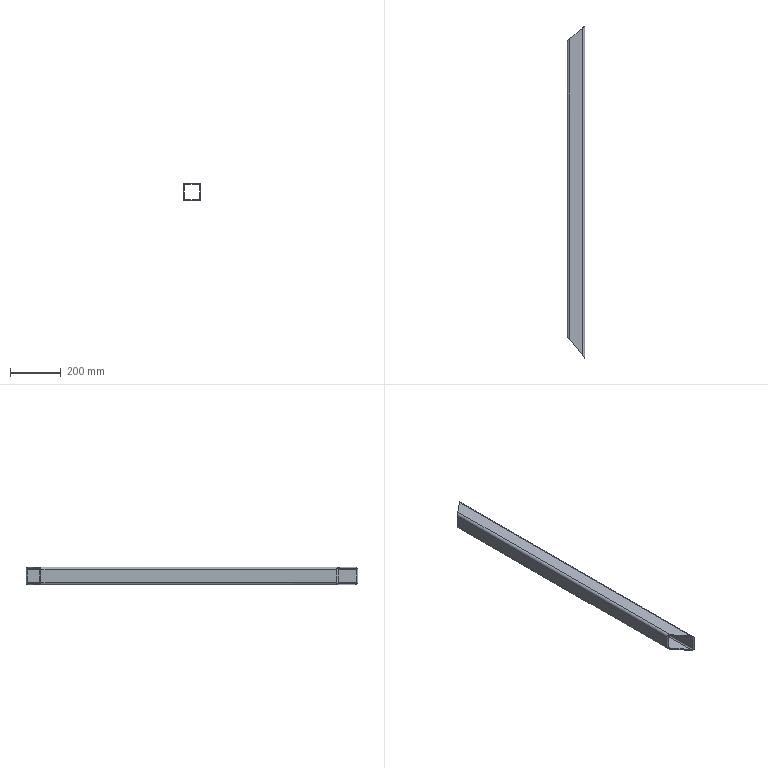Part | SolidWorks | features ICE 1, WeldMemberFeat 1, WeldmentFeature 1 | 1 solid | 18 faces | box 70 x 1302 x 70 mm | volume 1520953 mm3 | plane 10 | cylinder 8 | commonest cylinder face diameters 10 x4 20 x4
STEP:
#1=CARTESIAN_POINT('',(35.,0.,25.));
#2=VERTEX_POINT('',#1);
#3=CARTESIAN_POINT('',(35.,0.,-25.));
#4=VERTEX_POINT('',#3);
#5=CARTESIAN_POINT('',(35.,0.,-25.));
#6=DIRECTION('',(0.,0.,-1.));
#7=VECTOR('',#6,1000.);
#8=LINE('',#5,#7);
#9=EDGE_CURVE('',#2,#4,#8,.T.);
#10=ORIENTED_EDGE('',*,*,#9,.T.);
#11=CARTESIAN_POINT('',(35.,1302.,-25.));
#12=VERTEX_POINT('',#11);
#13=CARTESIAN_POINT('',(35.,1302.,-25.));
#14=DIRECTION('',(0.,-1.,0.));
#15=VECTOR('',#14,1000.);
#16=LINE('',#13,#15);
#17=EDGE_CURVE('',#12,#4,#16,.T.);
#18=ORIENTED_EDGE('',*,*,#17,.F.);
#19=CARTESIAN_POINT('',(35.,1302.,25.));
#20=VERTEX_POINT('',#19);
#21=CARTESIAN_POINT('',(35.,1302.,-25.));
#22=DIRECTION('',(0.,0.,-1.));
#23=VECTOR('',#22,1000.);
#24=LINE('',#21,#23);
#25=EDGE_CURVE('',#20,#12,#24,.T.);
#26=ORIENTED_EDGE('',*,*,#25,.F.);
#27=CARTESIAN_POINT('',(35.,1302.,25.));
#28=DIRECTION('',(0.,-1.,0.));
#29=VECTOR('',#28,1000.);
#30=LINE('',#27,#29);
#31=EDGE_CURVE('',#20,#2,#30,.T.);
#32=ORIENTED_EDGE('',*,*,#31,.T.);
#33=EDGE_LOOP('',(#10,#18,#26,#32));
#34=FACE_OUTER_BOUND('',#33,.T.);
#35=CARTESIAN_POINT('',(35.,1302.,-25.));
#36=DIRECTION('',(-1.,0.,0.));
#37=DIRECTION('',(0.,0.,1.));
#38=AXIS2_PLACEMENT_3D('',#35,#36,#37);
#39=PLANE('',#38);
#40=ADVANCED_FACE('',(#34),#39,.F.);
#41=CARTESIAN_POINT('',(-35.,1243.247,25.));
#42=VERTEX_POINT('',#41);
#43=CARTESIAN_POINT('',(-35.,83.4,25.));
#44=VERTEX_POINT('',#43);
#45=CARTESIAN_POINT('',(-35.,1302.,25.));
#46=DIRECTION('',(0.,-1.,0.));
#47=VECTOR('',#46,1000.);
#48=LINE('',#45,#47);
#49=EDGE_CURVE('',#42,#44,#48,.T.);
#50=ORIENTED_EDGE('',*,*,#49,.F.);
#51=CARTESIAN_POINT('',(-35.,1243.247,-25.));
#52=VERTEX_POINT('',#51);
#53=CARTESIAN_POINT('',(-35.,1243.247,-35.));
#54=DIRECTION('',(0.,0.,1.));
#55=VECTOR('',#54,1000.);
#56=LINE('',#53,#55);
#57=EDGE_CURVE('',#52,#42,#56,.T.);
#58=ORIENTED_EDGE('',*,*,#57,.F.);
#59=CARTESIAN_POINT('',(-35.,83.4,-25.));
#60=VERTEX_POINT('',#59);
#61=CARTESIAN_POINT('',(-35.,1302.,-25.));
#62=DIRECTION('',(0.,-1.,0.));
#63=VECTOR('',#62,1000.);
#64=LINE('',#61,#63);
#65=EDGE_CURVE('',#52,#60,#64,.T.);
#66=ORIENTED_EDGE('',*,*,#65,.T.);
#67=CARTESIAN_POINT('',(-35.,83.4,-35.));
#68=DIRECTION('',(0.,0.,1.));
#69=VECTOR('',#68,1000.);
#70=LINE('',#67,#69);
#71=EDGE_CURVE('',#60,#44,#70,.T.);
#72=ORIENTED_EDGE('',*,*,#71,.T.);
#73=EDGE_LOOP('',(#50,#58,#66,#72));
#74=FACE_OUTER_BOUND('',#73,.T.);
#75=CARTESIAN_POINT('',(-35.,1302.,25.));
#76=DIRECTION('',(1.,0.,0.));
#77=DIRECTION('',(0.,0.,-1.));
#78=AXIS2_PLACEMENT_3D('',#75,#76,#77);
#79=PLANE('',#78);
#80=ADVANCED_FACE('',(#74),#79,.F.);
#81=ORIENTED_EDGE('',*,*,#65,.F.);
#82=CARTESIAN_POINT('',(-25.,1251.64,-35.));
#83=VERTEX_POINT('',#82);
#84=CARTESIAN_POINT('',(-35.,1243.247,-25.));
#85=CARTESIAN_POINT('',(-35.,1243.247,-30.858));
#86=CARTESIAN_POINT('',(-30.858,1246.724,-35.));
#87=CARTESIAN_POINT('',(-25.,1251.64,-35.));
#88=(BOUNDED_CURVE()B_SPLINE_CURVE(3,(#84,#85,#86,#87),.UNSPECIFIED.,.F.,.F.)B_SPLINE_CURVE_WITH_KNOTS((4,4),(0.,1.571),.UNSPECIFIED.)CURVE()GEOMETRIC_REPRESENTATION_ITEM()RATIONAL_B_SPLINE_CURVE((1.,0.8047,0.8047,1.))REPRESENTATION_ITEM(''));
#89=EDGE_CURVE('',#52,#83,#88,.T.);
#90=ORIENTED_EDGE('',*,*,#89,.T.);
#91=CARTESIAN_POINT('',(-25.,71.486,-35.));
#92=VERTEX_POINT('',#91);
#93=CARTESIAN_POINT('',(-25.,1302.,-35.));
#94=DIRECTION('',(0.,-1.,0.));
#95=VECTOR('',#94,1000.);
#96=LINE('',#93,#95);
#97=EDGE_CURVE('',#83,#92,#96,.T.);
#98=ORIENTED_EDGE('',*,*,#97,.T.);
#99=CARTESIAN_POINT('',(-25.,71.486,-35.));
#100=CARTESIAN_POINT('',(-30.858,78.465,-35.));
#101=CARTESIAN_POINT('',(-35.,83.4,-30.858));
#102=CARTESIAN_POINT('',(-35.,83.4,-25.));
#103=(BOUNDED_CURVE()B_SPLINE_CURVE(3,(#99,#100,#101,#102),.UNSPECIFIED.,.F.,.F.)B_SPLINE_CURVE_WITH_KNOTS((4,4),(1.571,3.142),.UNSPECIFIED.)CURVE()GEOMETRIC_REPRESENTATION_ITEM()RATIONAL_B_SPLINE_CURVE((1.,0.8047,0.8047,1.))REPRESENTATION_ITEM(''));
#104=EDGE_CURVE('',#92,#60,#103,.T.);
#105=ORIENTED_EDGE('',*,*,#104,.T.);
#106=EDGE_LOOP('',(#81,#90,#98,#105));
#107=FACE_OUTER_BOUND('',#106,.T.);
#108=CARTESIAN_POINT('',(-25.,1302.,-25.));
#109=DIRECTION('',(0.,-1.,0.));
#110=DIRECTION('',(0.,0.,-1.));
#111=AXIS2_PLACEMENT_3D('',#108,#109,#110);
#112=CYLINDRICAL_SURFACE('',#111,10.);
#113=ADVANCED_FACE('',(#107),#112,.T.);
#114=ORIENTED_EDGE('',*,*,#97,.F.);
#115=CARTESIAN_POINT('',(25.,1293.607,-35.));
#116=VERTEX_POINT('',#115);
#117=CARTESIAN_POINT('',(35.,1302.,-35.));
#118=DIRECTION('',(0.766,0.6429,0.));
#119=VECTOR('',#118,1000.);
#120=LINE('',#117,#119);
#121=EDGE_CURVE('',#83,#116,#120,.T.);
#122=ORIENTED_EDGE('',*,*,#121,.T.);
#123=CARTESIAN_POINT('',(25.,11.914,-35.));
#124=VERTEX_POINT('',#123);
#125=CARTESIAN_POINT('',(25.,1302.,-35.));
#126=DIRECTION('',(0.,-1.,0.));
#127=VECTOR('',#126,1000.);
#128=LINE('',#125,#127);
#129=EDGE_CURVE('',#116,#124,#128,.T.);
#130=ORIENTED_EDGE('',*,*,#129,.T.);
#131=CARTESIAN_POINT('',(-35.,83.4,-35.));
#132=DIRECTION('',(-0.6429,0.766,0.));
#133=VECTOR('',#132,1000.);
#134=LINE('',#131,#133);
#135=EDGE_CURVE('',#124,#92,#134,.T.);
#136=ORIENTED_EDGE('',*,*,#135,.T.);
#137=EDGE_LOOP('',(#114,#122,#130,#136));
#138=FACE_OUTER_BOUND('',#137,.T.);
#139=CARTESIAN_POINT('',(25.,1302.,-35.));
#140=DIRECTION('',(0.,0.,1.));
#141=DIRECTION('',(1.,0.,0.));
#142=AXIS2_PLACEMENT_3D('',#139,#140,#141);
#143=PLANE('',#142);
#144=ADVANCED_FACE('',(#138),#143,.F.);
#145=ORIENTED_EDGE('',*,*,#129,.F.);
#146=CARTESIAN_POINT('',(25.,1293.607,-35.));
#147=CARTESIAN_POINT('',(30.858,1298.523,-35.));
#148=CARTESIAN_POINT('',(35.,1302.,-30.858));
#149=CARTESIAN_POINT('',(35.,1302.,-25.));
#150=(BOUNDED_CURVE()B_SPLINE_CURVE(3,(#146,#147,#148,#149),.UNSPECIFIED.,.F.,.F.)B_SPLINE_CURVE_WITH_KNOTS((4,4),(1.571,3.142),.UNSPECIFIED.)CURVE()GEOMETRIC_REPRESENTATION_ITEM()RATIONAL_B_SPLINE_CURVE((1.,0.8047,0.8047,1.))REPRESENTATION_ITEM(''));
#151=EDGE_CURVE('',#116,#12,#150,.T.);
#152=ORIENTED_EDGE('',*,*,#151,.T.);
#153=ORIENTED_EDGE('',*,*,#17,.T.);
#154=CARTESIAN_POINT('',(35.,0.,-25.));
#155=CARTESIAN_POINT('',(35.,0.,-30.858));
#156=CARTESIAN_POINT('',(30.858,4.935,-35.));
#157=CARTESIAN_POINT('',(25.,11.914,-35.));
#158=(BOUNDED_CURVE()B_SPLINE_CURVE(3,(#154,#155,#156,#157),.UNSPECIFIED.,.F.,.F.)B_SPLINE_CURVE_WITH_KNOTS((4,4),(0.,1.571),.UNSPECIFIED.)CURVE()GEOMETRIC_REPRESENTATION_ITEM()RATIONAL_B_SPLINE_CURVE((1.,0.8047,0.8047,1.))REPRESENTATION_ITEM(''));
#159=EDGE_CURVE('',#4,#124,#158,.T.);
#160=ORIENTED_EDGE('',*,*,#159,.T.);
#161=EDGE_LOOP('',(#145,#152,#153,#160));
#162=FACE_OUTER_BOUND('',#161,.T.);
#163=CARTESIAN_POINT('',(25.,1302.,-25.));
#164=DIRECTION('',(0.,-1.,0.));
#165=DIRECTION('',(0.,0.,-1.));
#166=AXIS2_PLACEMENT_3D('',#163,#164,#165);
#167=CYLINDRICAL_SURFACE('',#166,10.);
#168=ADVANCED_FACE('',(#162),#167,.T.);
#169=ORIENTED_EDGE('',*,*,#31,.F.);
#170=CARTESIAN_POINT('',(25.,1293.607,35.));
#171=VERTEX_POINT('',#170);
#172=CARTESIAN_POINT('',(35.,1302.,25.));
#173=CARTESIAN_POINT('',(35.,1302.,30.858));
#174=CARTESIAN_POINT('',(30.858,1298.523,35.));
#175=CARTESIAN_POINT('',(25.,1293.607,35.));
#176=(BOUNDED_CURVE()B_SPLINE_CURVE(3,(#172,#173,#174,#175),.UNSPECIFIED.,.F.,.F.)B_SPLINE_CURVE_WITH_KNOTS((4,4),(3.142,4.712),.UNSPECIFIED.)CURVE()GEOMETRIC_REPRESENTATION_ITEM()RATIONAL_B_SPLINE_CURVE((1.,0.8047,0.8047,1.))REPRESENTATION_ITEM(''));
#177=EDGE_CURVE('',#20,#171,#176,.T.);
#178=ORIENTED_EDGE('',*,*,#177,.T.);
#179=CARTESIAN_POINT('',(25.,11.914,35.));
#180=VERTEX_POINT('',#179);
#181=CARTESIAN_POINT('',(25.,1302.,35.));
#182=DIRECTION('',(0.,-1.,0.));
#183=VECTOR('',#182,1000.);
#184=LINE('',#181,#183);
#185=EDGE_CURVE('',#171,#180,#184,.T.);
#186=ORIENTED_EDGE('',*,*,#185,.T.);
#187=CARTESIAN_POINT('',(25.,11.914,35.));
#188=CARTESIAN_POINT('',(30.858,4.935,35.));
#189=CARTESIAN_POINT('',(35.,0.,30.858));
#190=CARTESIAN_POINT('',(35.,0.,25.));
#191=(BOUNDED_CURVE()B_SPLINE_CURVE(3,(#187,#188,#189,#190),.UNSPECIFIED.,.F.,.F.)B_SPLINE_CURVE_WITH_KNOTS((4,4),(4.712,6.283),.UNSPECIFIED.)CURVE()GEOMETRIC_REPRESENTATION_ITEM()RATIONAL_B_SPLINE_CURVE((1.,0.8047,0.8047,1.))REPRESENTATION_ITEM(''));
#192=EDGE_CURVE('',#180,#2,#191,.T.);
#193=ORIENTED_EDGE('',*,*,#192,.T.);
#194=EDGE_LOOP('',(#169,#178,#186,#193));
#195=FACE_OUTER_BOUND('',#194,.T.);
#196=CARTESIAN_POINT('',(25.,1302.,25.));
#197=DIRECTION('',(0.,-1.,0.));
#198=DIRECTION('',(0.,0.,-1.));
#199=AXIS2_PLACEMENT_3D('',#196,#197,#198);
#200=CYLINDRICAL_SURFACE('',#199,10.);
#201=ADVANCED_FACE('',(#195),#200,.T.);
#202=ORIENTED_EDGE('',*,*,#185,.F.);
#203=CARTESIAN_POINT('',(-25.,1251.64,35.));
#204=VERTEX_POINT('',#203);
#205=CARTESIAN_POINT('',(-0.2015,1272.454,35.));
#206=DIRECTION('',(-0.766,-0.6429,0.));
#207=VECTOR('',#206,1000.);
#208=LINE('',#205,#207);
#209=EDGE_CURVE('',#171,#204,#208,.T.);
#210=ORIENTED_EDGE('',*,*,#209,.T.);
#211=CARTESIAN_POINT('',(-25.,71.486,35.));
#212=VERTEX_POINT('',#211);
#213=CARTESIAN_POINT('',(-25.,1302.,35.));
#214=DIRECTION('',(0.,-1.,0.));
#215=VECTOR('',#214,1000.);
#216=LINE('',#213,#215);
#217=EDGE_CURVE('',#204,#212,#216,.T.);
#218=ORIENTED_EDGE('',*,*,#217,.T.);
#219=CARTESIAN_POINT('',(-630.939,793.418,35.));
#220=DIRECTION('',(0.6429,-0.766,0.));
#221=VECTOR('',#220,1000.);
#222=LINE('',#219,#221);
#223=EDGE_CURVE('',#212,#180,#222,.T.);
#224=ORIENTED_EDGE('',*,*,#223,.T.);
#225=EDGE_LOOP('',(#202,#210,#218,#224));
#226=FACE_OUTER_BOUND('',#225,.T.);
#227=CARTESIAN_POINT('',(-25.,1302.,35.));
#228=DIRECTION('',(0.,0.,-1.));
#229=DIRECTION('',(-1.,0.,0.));
#230=AXIS2_PLACEMENT_3D('',#227,#228,#229);
#231=PLANE('',#230);
#232=ADVANCED_FACE('',(#226),#231,.F.);
#233=ORIENTED_EDGE('',*,*,#217,.F.);
#234=CARTESIAN_POINT('',(-25.,1251.64,35.));
#235=CARTESIAN_POINT('',(-30.858,1246.724,35.));
#236=CARTESIAN_POINT('',(-35.,1243.247,30.858));
#237=CARTESIAN_POINT('',(-35.,1243.247,25.));
#238=(BOUNDED_CURVE()B_SPLINE_CURVE(3,(#234,#235,#236,#237),.UNSPECIFIED.,.F.,.T.)B_SPLINE_CURVE_WITH_KNOTS((4,4),(4.712,6.283),.UNSPECIFIED.)CURVE()GEOMETRIC_REPRESENTATION_ITEM()RATIONAL_B_SPLINE_CURVE((1.,0.8047,0.8047,1.))REPRESENTATION_ITEM(''));
#239=EDGE_CURVE('',#204,#42,#238,.T.);
#240=ORIENTED_EDGE('',*,*,#239,.T.);
#241=ORIENTED_EDGE('',*,*,#49,.T.);
#242=CARTESIAN_POINT('',(-35.,83.4,25.));
#243=CARTESIAN_POINT('',(-35.,83.4,30.858));
#244=CARTESIAN_POINT('',(-30.858,78.465,35.));
#245=CARTESIAN_POINT('',(-25.,71.486,35.));
#246=(BOUNDED_CURVE()B_SPLINE_CURVE(3,(#242,#243,#244,#245),.UNSPECIFIED.,.F.,.T.)B_SPLINE_CURVE_WITH_KNOTS((4,4),(3.142,4.712),.UNSPECIFIED.)CURVE()GEOMETRIC_REPRESENTATION_ITEM()RATIONAL_B_SPLINE_CURVE((1.,0.8047,0.8047,1.))REPRESENTATION_ITEM(''));
#247=EDGE_CURVE('',#44,#212,#246,.T.);
#248=ORIENTED_EDGE('',*,*,#247,.T.);
#249=EDGE_LOOP('',(#233,#240,#241,#248));
#250=FACE_OUTER_BOUND('',#249,.T.);
#251=CARTESIAN_POINT('',(-25.,1302.,25.));
#252=DIRECTION('',(0.,-1.,0.));
#253=DIRECTION('',(0.,0.,-1.));
#254=AXIS2_PLACEMENT_3D('',#251,#252,#253);
#255=CYLINDRICAL_SURFACE('',#254,10.);
#256=ADVANCED_FACE('',(#250),#255,.T.);
#257=CARTESIAN_POINT('',(25.,11.914,30.));
#258=VERTEX_POINT('',#257);
#259=CARTESIAN_POINT('',(30.,5.957,25.));
#260=VERTEX_POINT('',#259);
#261=CARTESIAN_POINT('',(25.,11.914,30.));
#262=CARTESIAN_POINT('',(27.929,8.425,30.));
#263=CARTESIAN_POINT('',(30.,5.957,27.929));
#264=CARTESIAN_POINT('',(30.,5.957,25.));
#265=(BOUNDED_CURVE()B_SPLINE_CURVE(3,(#261,#262,#263,#264),.UNSPECIFIED.,.F.,.F.)B_SPLINE_CURVE_WITH_KNOTS((4,4),(4.712,6.283),.UNSPECIFIED.)CURVE()GEOMETRIC_REPRESENTATION_ITEM()RATIONAL_B_SPLINE_CURVE((1.,0.8047,0.8047,1.))REPRESENTATION_ITEM(''));
#266=EDGE_CURVE('',#258,#260,#265,.T.);
#267=ORIENTED_EDGE('',*,*,#266,.T.);
#268=CARTESIAN_POINT('',(30.,5.957,-25.));
#269=VERTEX_POINT('',#268);
#270=CARTESIAN_POINT('',(30.,5.957,-25.));
#271=DIRECTION('',(0.,0.,-1.));
#272=VECTOR('',#271,1000.);
#273=LINE('',#270,#272);
#274=EDGE_CURVE('',#260,#269,#273,.T.);
#275=ORIENTED_EDGE('',*,*,#274,.T.);
#276=CARTESIAN_POINT('',(25.,11.914,-30.));
#277=VERTEX_POINT('',#276);
#278=CARTESIAN_POINT('',(30.,5.957,-25.));
#279=CARTESIAN_POINT('',(30.,5.957,-27.929));
#280=CARTESIAN_POINT('',(27.929,8.425,-30.));
#281=CARTESIAN_POINT('',(25.,11.914,-30.));
#282=(BOUNDED_CURVE()B_SPLINE_CURVE(3,(#278,#279,#280,#281),.UNSPECIFIED.,.F.,.F.)B_SPLINE_CURVE_WITH_KNOTS((4,4),(0.,1.571),.UNSPECIFIED.)CURVE()GEOMETRIC_REPRESENTATION_ITEM()RATIONAL_B_SPLINE_CURVE((1.,0.8047,0.8047,1.))REPRESENTATION_ITEM(''));
#283=EDGE_CURVE('',#269,#277,#282,.T.);
#284=ORIENTED_EDGE('',*,*,#283,.T.);
#285=CARTESIAN_POINT('',(-25.,71.486,-30.));
#286=VERTEX_POINT('',#285);
#287=CARTESIAN_POINT('',(-610.273,768.797,-30.));
#288=DIRECTION('',(-0.6429,0.766,0.));
#289=VECTOR('',#288,1000.);
#290=LINE('',#287,#289);
#291=EDGE_CURVE('',#277,#286,#290,.T.);
#292=ORIENTED_EDGE('',*,*,#291,.T.);
#293=CARTESIAN_POINT('',(-30.,77.443,-25.));
#294=VERTEX_POINT('',#293);
#295=CARTESIAN_POINT('',(-25.,71.486,-30.));
#296=CARTESIAN_POINT('',(-27.929,74.975,-30.));
#297=CARTESIAN_POINT('',(-30.,77.443,-27.929));
#298=CARTESIAN_POINT('',(-30.,77.443,-25.));
#299=(BOUNDED_CURVE()B_SPLINE_CURVE(3,(#295,#296,#297,#298),.UNSPECIFIED.,.F.,.F.)B_SPLINE_CURVE_WITH_KNOTS((4,4),(1.571,3.142),.UNSPECIFIED.)CURVE()GEOMETRIC_REPRESENTATION_ITEM()RATIONAL_B_SPLINE_CURVE((1.,0.8047,0.8047,1.))REPRESENTATION_ITEM(''));
#300=EDGE_CURVE('',#286,#294,#299,.T.);
#301=ORIENTED_EDGE('',*,*,#300,.T.);
#302=CARTESIAN_POINT('',(-30.,77.443,25.));
#303=VERTEX_POINT('',#302);
#304=CARTESIAN_POINT('',(-30.,77.443,25.));
#305=DIRECTION('',(0.,0.,1.));
#306=VECTOR('',#305,1000.);
#307=LINE('',#304,#306);
#308=EDGE_CURVE('',#294,#303,#307,.T.);
#309=ORIENTED_EDGE('',*,*,#308,.T.);
#310=CARTESIAN_POINT('',(-25.,71.486,30.));
#311=VERTEX_POINT('',#310);
#312=CARTESIAN_POINT('',(-30.,77.443,25.));
#313=CARTESIAN_POINT('',(-30.,77.443,27.929));
#314=CARTESIAN_POINT('',(-27.929,74.975,30.));
#315=CARTESIAN_POINT('',(-25.,71.486,30.));
#316=(BOUNDED_CURVE()B_SPLINE_CURVE(3,(#312,#313,#314,#315),.UNSPECIFIED.,.F.,.T.)B_SPLINE_CURVE_WITH_KNOTS((4,4),(3.142,4.712),.UNSPECIFIED.)CURVE()GEOMETRIC_REPRESENTATION_ITEM()RATIONAL_B_SPLINE_CURVE((1.,0.8047,0.8047,1.))REPRESENTATION_ITEM(''));
#317=EDGE_CURVE('',#303,#311,#316,.T.);
#318=ORIENTED_EDGE('',*,*,#317,.T.);
#319=CARTESIAN_POINT('',(-630.939,793.418,30.));
#320=DIRECTION('',(0.6429,-0.766,0.));
#321=VECTOR('',#320,1000.);
#322=LINE('',#319,#321);
#323=EDGE_CURVE('',#311,#258,#322,.T.);
#324=ORIENTED_EDGE('',*,*,#323,.T.);
#325=EDGE_LOOP('',(#267,#275,#284,#292,#301,#309,#318,#324));
#326=FACE_BOUND('',#325,.T.);
#327=ORIENTED_EDGE('',*,*,#71,.F.);
#328=ORIENTED_EDGE('',*,*,#104,.F.);
#329=ORIENTED_EDGE('',*,*,#135,.F.);
#330=ORIENTED_EDGE('',*,*,#159,.F.);
#331=ORIENTED_EDGE('',*,*,#9,.F.);
#332=ORIENTED_EDGE('',*,*,#192,.F.);
#333=ORIENTED_EDGE('',*,*,#223,.F.);
#334=ORIENTED_EDGE('',*,*,#247,.F.);
#335=EDGE_LOOP('',(#327,#328,#329,#330,#331,#332,#333,#334));
#336=FACE_OUTER_BOUND('',#335,.T.);
#337=CARTESIAN_POINT('',(-35.,83.4,-35.));
#338=DIRECTION('',(0.766,0.6429,0.));
#339=DIRECTION('',(-0.6429,0.766,0.));
#340=AXIS2_PLACEMENT_3D('',#337,#338,#339);
#341=PLANE('',#340);
#342=ADVANCED_FACE('',(#326,#336),#341,.F.);
#343=CARTESIAN_POINT('',(30.,1297.803,25.));
#344=VERTEX_POINT('',#343);
#345=CARTESIAN_POINT('',(25.,1293.607,30.));
#346=VERTEX_POINT('',#345);
#347=CARTESIAN_POINT('',(30.,1297.803,25.));
#348=CARTESIAN_POINT('',(30.,1297.803,27.929));
#349=CARTESIAN_POINT('',(27.929,1296.065,30.));
#350=CARTESIAN_POINT('',(25.,1293.607,30.));
#351=(BOUNDED_CURVE()B_SPLINE_CURVE(3,(#347,#348,#349,#350),.UNSPECIFIED.,.F.,.F.)B_SPLINE_CURVE_WITH_KNOTS((4,4),(3.142,4.712),.UNSPECIFIED.)CURVE()GEOMETRIC_REPRESENTATION_ITEM()RATIONAL_B_SPLINE_CURVE((1.,0.8047,0.8047,1.))REPRESENTATION_ITEM(''));
#352=EDGE_CURVE('',#344,#346,#351,.T.);
#353=ORIENTED_EDGE('',*,*,#352,.T.);
#354=CARTESIAN_POINT('',(-25.,1251.64,30.));
#355=VERTEX_POINT('',#354);
#356=CARTESIAN_POINT('',(-0.2015,1272.454,30.));
#357=DIRECTION('',(-0.766,-0.6429,0.));
#358=VECTOR('',#357,1000.);
#359=LINE('',#356,#358);
#360=EDGE_CURVE('',#346,#355,#359,.T.);
#361=ORIENTED_EDGE('',*,*,#360,.T.);
#362=CARTESIAN_POINT('',(-30.,1247.444,25.));
#363=VERTEX_POINT('',#362);
#364=CARTESIAN_POINT('',(-25.,1251.64,30.));
#365=CARTESIAN_POINT('',(-27.929,1249.182,30.));
#366=CARTESIAN_POINT('',(-30.,1247.444,27.929));
#367=CARTESIAN_POINT('',(-30.,1247.444,25.));
#368=(BOUNDED_CURVE()B_SPLINE_CURVE(3,(#364,#365,#366,#367),.UNSPECIFIED.,.F.,.F.)B_SPLINE_CURVE_WITH_KNOTS((4,4),(4.712,6.283),.UNSPECIFIED.)CURVE()GEOMETRIC_REPRESENTATION_ITEM()RATIONAL_B_SPLINE_CURVE((1.,0.8047,0.8047,1.))REPRESENTATION_ITEM(''));
#369=EDGE_CURVE('',#355,#363,#368,.T.);
#370=ORIENTED_EDGE('',*,*,#369,.T.);
#371=CARTESIAN_POINT('',(-30.,1247.444,-25.));
#372=VERTEX_POINT('',#371);
#373=CARTESIAN_POINT('',(-30.,1247.444,25.));
#374=DIRECTION('',(0.,0.,-1.));
#375=VECTOR('',#374,1000.);
#376=LINE('',#373,#375);
#377=EDGE_CURVE('',#363,#372,#376,.T.);
#378=ORIENTED_EDGE('',*,*,#377,.T.);
#379=CARTESIAN_POINT('',(-25.,1251.64,-30.));
#380=VERTEX_POINT('',#379);
#381=CARTESIAN_POINT('',(-30.,1247.444,-25.));
#382=CARTESIAN_POINT('',(-30.,1247.444,-27.929));
#383=CARTESIAN_POINT('',(-27.929,1249.182,-30.));
#384=CARTESIAN_POINT('',(-25.,1251.64,-30.));
#385=(BOUNDED_CURVE()B_SPLINE_CURVE(3,(#381,#382,#383,#384),.UNSPECIFIED.,.F.,.F.)B_SPLINE_CURVE_WITH_KNOTS((4,4),(0.,1.571),.UNSPECIFIED.)CURVE()GEOMETRIC_REPRESENTATION_ITEM()RATIONAL_B_SPLINE_CURVE((1.,0.8047,0.8047,1.))REPRESENTATION_ITEM(''));
#386=EDGE_CURVE('',#372,#380,#385,.T.);
#387=ORIENTED_EDGE('',*,*,#386,.T.);
#388=CARTESIAN_POINT('',(25.,1293.607,-30.));
#389=VERTEX_POINT('',#388);
#390=CARTESIAN_POINT('',(29.133,1297.076,-30.));
#391=DIRECTION('',(0.766,0.6429,0.));
#392=VECTOR('',#391,1000.);
#393=LINE('',#390,#392);
#394=EDGE_CURVE('',#380,#389,#393,.T.);
#395=ORIENTED_EDGE('',*,*,#394,.T.);
#396=CARTESIAN_POINT('',(30.,1297.803,-25.));
#397=VERTEX_POINT('',#396);
#398=CARTESIAN_POINT('',(25.,1293.607,-30.));
#399=CARTESIAN_POINT('',(27.929,1296.065,-30.));
#400=CARTESIAN_POINT('',(30.,1297.803,-27.929));
#401=CARTESIAN_POINT('',(30.,1297.803,-25.));
#402=(BOUNDED_CURVE()B_SPLINE_CURVE(3,(#398,#399,#400,#401),.UNSPECIFIED.,.F.,.F.)B_SPLINE_CURVE_WITH_KNOTS((4,4),(1.571,3.142),.UNSPECIFIED.)CURVE()GEOMETRIC_REPRESENTATION_ITEM()RATIONAL_B_SPLINE_CURVE((1.,0.8047,0.8047,1.))REPRESENTATION_ITEM(''));
#403=EDGE_CURVE('',#389,#397,#402,.T.);
#404=ORIENTED_EDGE('',*,*,#403,.T.);
#405=CARTESIAN_POINT('',(30.,1297.803,-25.));
#406=DIRECTION('',(0.,0.,1.));
#407=VECTOR('',#406,1000.);
#408=LINE('',#405,#407);
#409=EDGE_CURVE('',#397,#344,#408,.T.);
#410=ORIENTED_EDGE('',*,*,#409,.T.);
#411=EDGE_LOOP('',(#353,#361,#370,#378,#387,#395,#404,#410));
#412=FACE_BOUND('',#411,.T.);
#413=ORIENTED_EDGE('',*,*,#209,.F.);
#414=ORIENTED_EDGE('',*,*,#177,.F.);
#415=ORIENTED_EDGE('',*,*,#25,.T.);
#416=ORIENTED_EDGE('',*,*,#151,.F.);
#417=ORIENTED_EDGE('',*,*,#121,.F.);
#418=ORIENTED_EDGE('',*,*,#89,.F.);
#419=ORIENTED_EDGE('',*,*,#57,.T.);
#420=ORIENTED_EDGE('',*,*,#239,.F.);
#421=EDGE_LOOP('',(#413,#414,#415,#416,#417,#418,#419,#420));
#422=FACE_OUTER_BOUND('',#421,.T.);
#423=CARTESIAN_POINT('',(35.,1302.,-35.));
#424=DIRECTION('',(0.6429,-0.766,0.));
#425=DIRECTION('',(0.766,0.6429,0.));
#426=AXIS2_PLACEMENT_3D('',#423,#424,#425);
#427=PLANE('',#426);
#428=ADVANCED_FACE('',(#412,#422),#427,.F.);
#429=ORIENTED_EDGE('',*,*,#352,.F.);
#430=CARTESIAN_POINT('',(30.,1302.,25.));
#431=DIRECTION('',(0.,-1.,0.));
#432=VECTOR('',#431,1000.);
#433=LINE('',#430,#432);
#434=EDGE_CURVE('',#344,#260,#433,.T.);
#435=ORIENTED_EDGE('',*,*,#434,.T.);
#436=ORIENTED_EDGE('',*,*,#266,.F.);
#437=CARTESIAN_POINT('',(25.,1302.,30.));
#438=DIRECTION('',(0.,-1.,0.));
#439=VECTOR('',#438,1000.);
#440=LINE('',#437,#439);
#441=EDGE_CURVE('',#346,#258,#440,.T.);
#442=ORIENTED_EDGE('',*,*,#441,.F.);
#443=EDGE_LOOP('',(#429,#435,#436,#442));
#444=FACE_OUTER_BOUND('',#443,.T.);
#445=CARTESIAN_POINT('',(25.,1302.,25.));
#446=DIRECTION('',(0.,-1.,0.));
#447=DIRECTION('',(0.,0.,-1.));
#448=AXIS2_PLACEMENT_3D('',#445,#446,#447);
#449=CYLINDRICAL_SURFACE('',#448,5.);
#450=ADVANCED_FACE('',(#444),#449,.F.);
#451=ORIENTED_EDGE('',*,*,#360,.F.);
#452=ORIENTED_EDGE('',*,*,#441,.T.);
#453=ORIENTED_EDGE('',*,*,#323,.F.);
#454=CARTESIAN_POINT('',(-25.,1302.,30.));
#455=DIRECTION('',(0.,-1.,0.));
#456=VECTOR('',#455,1000.);
#457=LINE('',#454,#456);
#458=EDGE_CURVE('',#355,#311,#457,.T.);
#459=ORIENTED_EDGE('',*,*,#458,.F.);
#460=EDGE_LOOP('',(#451,#452,#453,#459));
#461=FACE_OUTER_BOUND('',#460,.T.);
#462=CARTESIAN_POINT('',(-25.,1302.,30.));
#463=DIRECTION('',(0.,0.,-1.));
#464=DIRECTION('',(-1.,0.,0.));
#465=AXIS2_PLACEMENT_3D('',#462,#463,#464);
#466=PLANE('',#465);
#467=ADVANCED_FACE('',(#461),#466,.T.);
#468=ORIENTED_EDGE('',*,*,#369,.F.);
#469=ORIENTED_EDGE('',*,*,#458,.T.);
#470=ORIENTED_EDGE('',*,*,#317,.F.);
#471=CARTESIAN_POINT('',(-30.,1302.,25.));
#472=DIRECTION('',(0.,-1.,0.));
#473=VECTOR('',#472,1000.);
#474=LINE('',#471,#473);
#475=EDGE_CURVE('',#363,#303,#474,.T.);
#476=ORIENTED_EDGE('',*,*,#475,.F.);
#477=EDGE_LOOP('',(#468,#469,#470,#476));
#478=FACE_OUTER_BOUND('',#477,.T.);
#479=CARTESIAN_POINT('',(-25.,1302.,25.));
#480=DIRECTION('',(0.,-1.,0.));
#481=DIRECTION('',(0.,0.,-1.));
#482=AXIS2_PLACEMENT_3D('',#479,#480,#481);
#483=CYLINDRICAL_SURFACE('',#482,5.);
#484=ADVANCED_FACE('',(#478),#483,.F.);
#485=ORIENTED_EDGE('',*,*,#377,.F.);
#486=ORIENTED_EDGE('',*,*,#475,.T.);
#487=ORIENTED_EDGE('',*,*,#308,.F.);
#488=CARTESIAN_POINT('',(-30.,1302.,-25.));
#489=DIRECTION('',(0.,-1.,0.));
#490=VECTOR('',#489,1000.);
#491=LINE('',#488,#490);
#492=EDGE_CURVE('',#372,#294,#491,.T.);
#493=ORIENTED_EDGE('',*,*,#492,.F.);
#494=EDGE_LOOP('',(#485,#486,#487,#493));
#495=FACE_OUTER_BOUND('',#494,.T.);
#496=CARTESIAN_POINT('',(-30.,1302.,25.));
#497=DIRECTION('',(1.,0.,0.));
#498=DIRECTION('',(0.,0.,-1.));
#499=AXIS2_PLACEMENT_3D('',#496,#497,#498);
#500=PLANE('',#499);
#501=ADVANCED_FACE('',(#495),#500,.T.);
#502=ORIENTED_EDGE('',*,*,#386,.F.);
#503=ORIENTED_EDGE('',*,*,#492,.T.);
#504=ORIENTED_EDGE('',*,*,#300,.F.);
#505=CARTESIAN_POINT('',(-25.,1302.,-30.));
#506=DIRECTION('',(0.,-1.,0.));
#507=VECTOR('',#506,1000.);
#508=LINE('',#505,#507);
#509=EDGE_CURVE('',#380,#286,#508,.T.);
#510=ORIENTED_EDGE('',*,*,#509,.F.);
#511=EDGE_LOOP('',(#502,#503,#504,#510));
#512=FACE_OUTER_BOUND('',#511,.T.);
#513=CARTESIAN_POINT('',(-25.,1302.,-25.));
#514=DIRECTION('',(0.,-1.,0.));
#515=DIRECTION('',(0.,0.,-1.));
#516=AXIS2_PLACEMENT_3D('',#513,#514,#515);
#517=CYLINDRICAL_SURFACE('',#516,5.);
#518=ADVANCED_FACE('',(#512),#517,.F.);
#519=ORIENTED_EDGE('',*,*,#394,.F.);
#520=ORIENTED_EDGE('',*,*,#509,.T.);
#521=ORIENTED_EDGE('',*,*,#291,.F.);
#522=CARTESIAN_POINT('',(25.,1302.,-30.));
#523=DIRECTION('',(0.,-1.,0.));
#524=VECTOR('',#523,1000.);
#525=LINE('',#522,#524);
#526=EDGE_CURVE('',#389,#277,#525,.T.);
#527=ORIENTED_EDGE('',*,*,#526,.F.);
#528=EDGE_LOOP('',(#519,#520,#521,#527));
#529=FACE_OUTER_BOUND('',#528,.T.);
#530=CARTESIAN_POINT('',(25.,1302.,-30.));
#531=DIRECTION('',(0.,0.,1.));
#532=DIRECTION('',(1.,0.,0.));
#533=AXIS2_PLACEMENT_3D('',#530,#531,#532);
#534=PLANE('',#533);
#535=ADVANCED_FACE('',(#529),#534,.T.);
#536=ORIENTED_EDGE('',*,*,#403,.F.);
#537=ORIENTED_EDGE('',*,*,#526,.T.);
#538=ORIENTED_EDGE('',*,*,#283,.F.);
#539=CARTESIAN_POINT('',(30.,1302.,-25.));
#540=DIRECTION('',(0.,-1.,0.));
#541=VECTOR('',#540,1000.);
#542=LINE('',#539,#541);
#543=EDGE_CURVE('',#397,#269,#542,.T.);
#544=ORIENTED_EDGE('',*,*,#543,.F.);
#545=EDGE_LOOP('',(#536,#537,#538,#544));
#546=FACE_OUTER_BOUND('',#545,.T.);
#547=CARTESIAN_POINT('',(25.,1302.,-25.));
#548=DIRECTION('',(0.,-1.,0.));
#549=DIRECTION('',(0.,0.,-1.));
#550=AXIS2_PLACEMENT_3D('',#547,#548,#549);
#551=CYLINDRICAL_SURFACE('',#550,5.);
#552=ADVANCED_FACE('',(#546),#551,.F.);
#553=ORIENTED_EDGE('',*,*,#409,.F.);
#554=ORIENTED_EDGE('',*,*,#543,.T.);
#555=ORIENTED_EDGE('',*,*,#274,.F.);
#556=ORIENTED_EDGE('',*,*,#434,.F.);
#557=EDGE_LOOP('',(#553,#554,#555,#556));
#558=FACE_OUTER_BOUND('',#557,.T.);
#559=CARTESIAN_POINT('',(30.,1302.,-25.));
#560=DIRECTION('',(-1.,0.,0.));
#561=DIRECTION('',(0.,0.,1.));
#562=AXIS2_PLACEMENT_3D('',#559,#560,#561);
#563=PLANE('',#562);
#564=ADVANCED_FACE('',(#558),#563,.T.);
#565=CLOSED_SHELL('',(#40,#80,#113,#144,#168,#201,#232,#256,#342,#428,#450,#467,#484,#501,#518,#535,#552,#564));
#566=MANIFOLD_SOLID_BREP('',#565);
#567=CARTESIAN_POINT('',(0.,0.,0.));
#568=DIRECTION('',(0.,0.,1.));
#569=DIRECTION('',(1.,0.,0.));
#570=AXIS2_PLACEMENT_3D('',#567,#568,#569);
#571=(LENGTH_UNIT()NAMED_UNIT(*)SI_UNIT(.MILLI.,.METRE.));
#572=UNCERTAINTY_MEASURE_WITH_UNIT(LENGTH_MEASURE(0.00001),#571,'','');
#573=(NAMED_UNIT(*)PLANE_ANGLE_UNIT()SI_UNIT($,.RADIAN.));
#574=(NAMED_UNIT(*)SI_UNIT($,.STERADIAN.)SOLID_ANGLE_UNIT());
#575=(GEOMETRIC_REPRESENTATION_CONTEXT(3)GLOBAL_UNCERTAINTY_ASSIGNED_CONTEXT((#572))GLOBAL_UNIT_ASSIGNED_CONTEXT((#571,#573,#574))REPRESENTATION_CONTEXT('',''));
#576=ADVANCED_BREP_SHAPE_REPRESENTATION('',(#566,#570),#575);